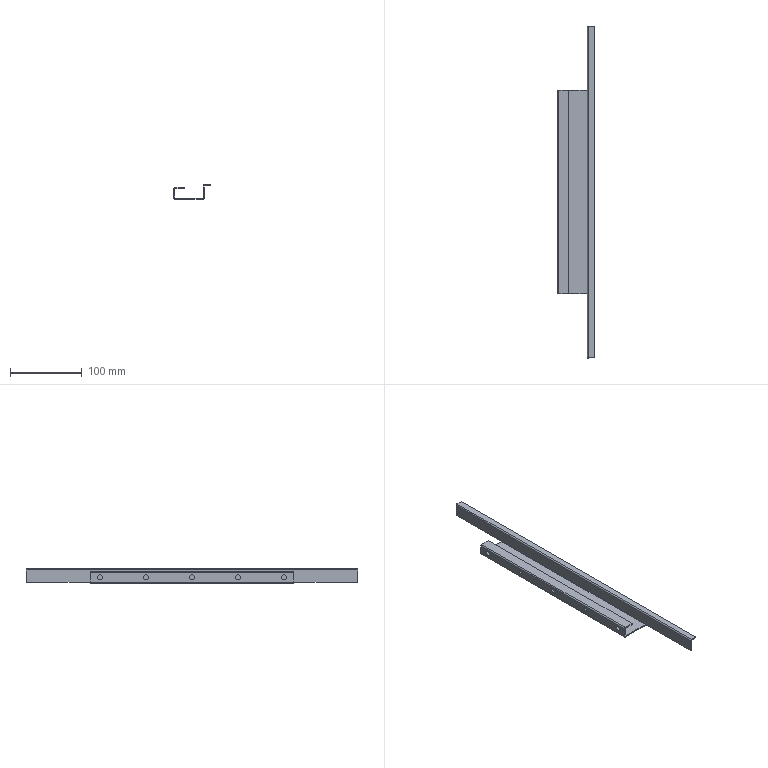Part | STEP file | HESS-408-70-15W-W-36-upper door glass inner frame 2 | 1 solid | 38 faces | box 51 x 462 x 20 mm | volume 47605 mm3 | cylinder 20 | plane 18 | commonest cylinder face diameters 7 x10 0.2 x4 3.2 x4 1 x2